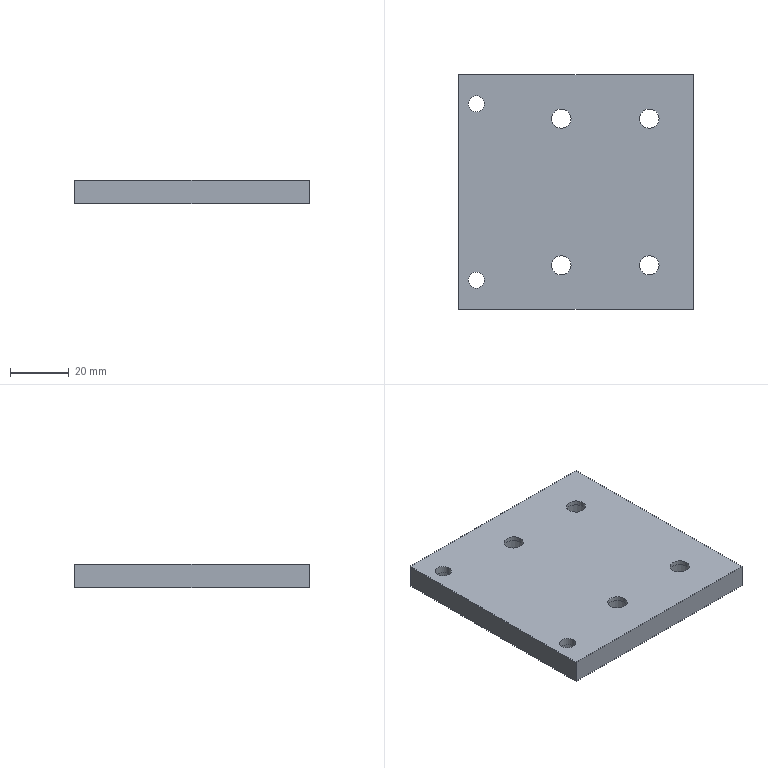Part | STEP file | CA-10-003Lift Stop Fixing Plate_Default | 1 solid | 36 faces | box 80 x 80 x 8 mm | volume 47659 mm3 | cylinder 24 | plane 12 | commonest cylinder face diameters 6.6 x8 11 x8 5.5 x4 9.5 x4